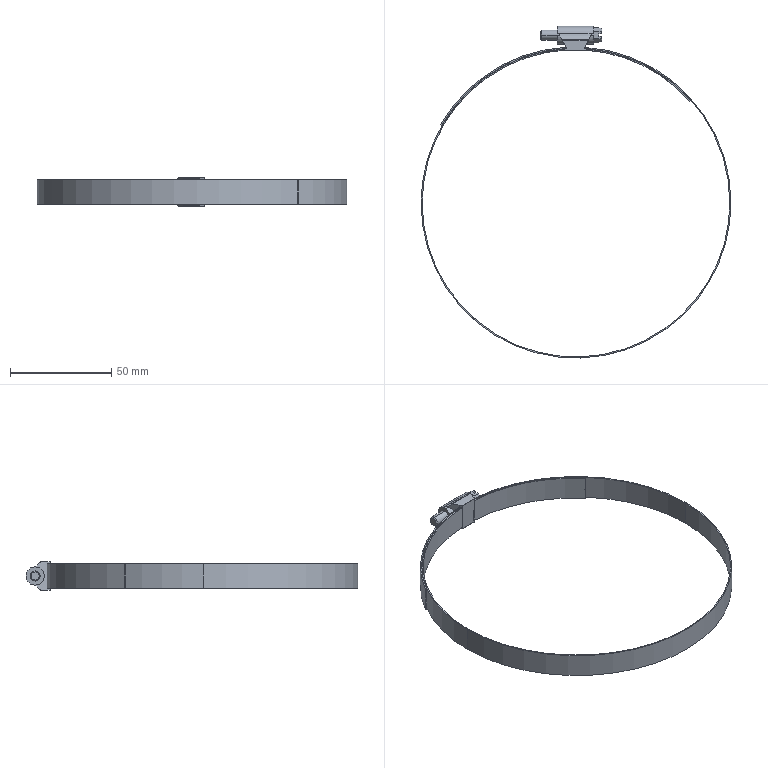Part | STEP file | _SPR_SPR-152_00 | 1 solid | 70 faces | box 153 x 163.967 x 14 mm | volume 6165 mm3 | plane 35 | cylinder 25 | cone 10 | commonest cylinder face diameters 9 x5 0.2 x2 1 x2 5 x2 151.025 x2 151.775 x2